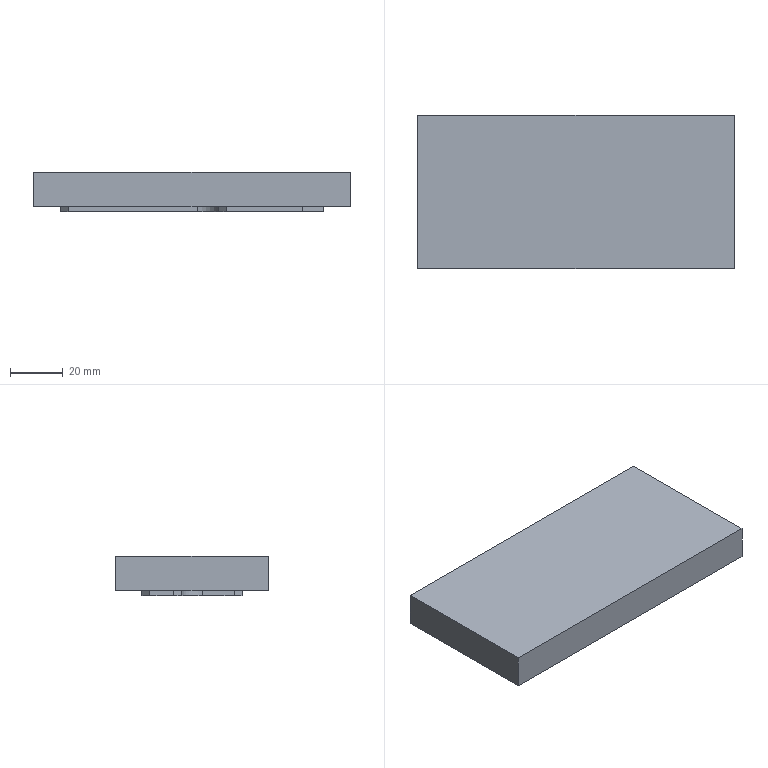NC program | NX | posted with a generic post | part box 120 x 58 x 15 mm
Lines 3611 to 3687 of 3687:
(11_COPY_COPY , TOOL : D6A45)
N7190 T01 M6
N7192 G54
N7194 G17 G0 G90 X30. Y0.741 S9500 M3
N7196 G43 Z30. H1
N7198 Z3.
N7200 G94 G1 Z-1. F1000.
N7202 X29.995
N7204 G3 X29.259 Y-0.005 R0.741
N7206 X30. Y0.741 R-0.741
N7208 X29.48 Y0.441 R0.6
N7210 G1 Z2.
N7212 G0 Z30.
N7214 X30. Y-14.791
N7216 Z3.
N7218 G1 Z-1.
N7220 G3 X44.791 Y0. R14.791
N7222 X30. Y14.791 R14.791
N7224 X29.209 Y14. R0.791
N7226 X30. Y13.209 R0.791
N7228 G2 X43.209 Y0. R13.209
N7230 X30. Y-13.209 R13.209
N7232 G3 X29.209 Y-14. R0.791
N7234 X30. Y-14.791 R0.791
N7236 X30.52 Y-14.491 R0.6
N7238 G1 Z2.
N7240 G0 Z30.
N7242 X6.042 Y13.081
N7244 Z2.
N7246 G1 Z-1.
N7248 X6.52 Y13.991
N7250 G3 X6. Y14.291 R0.6
N7252 G1 X-44.
N7254 G3 X-45.291 Y13. R1.291
N7256 X-44. Y11.709 R1.291
N7258 G1 X6.
N7260 G3 X7.291 Y13. R1.291
N7262 X6. Y14.291 R1.291
N7264 X5.48 Y13.991 R0.6
N7266 G1 X4.961 Y13.091
N7268 Z2.
N7270 G0 Z30.
N7272 X-47.921 Y20.952
N7274 Z2.
N7276 G1 Z-1.
N7278 X-47.52 Y20.259
N7280 G3 X-47.001 Y19.959 R0.6
N7282 G1 X42.001
N7284 G2 X42.677 Y19.678 R0.957
N7286 G1 X50.678 Y11.677
N7288 G2 X50.959 Y11. R0.957
N7290 G1 Y-11.
N7292 G2 X50.678 Y-11.677 R0.957
N7294 G1 X42.677 Y-19.678
N7296 G2 X42.001 Y-19.959 R0.957
N7298 G1 X12.999
N7300 G2 X12.323 Y-19.678 R0.957
N7302 G1 X9.322 Y-16.677
N7304 G2 X9.041 Y-16.001 R0.957
N7306 G1 Y-4.
N7308 G3 X2. Y3.041 R7.041
N7310 G1 X-47.001
N7312 G2 X-47.677 Y3.322 R0.957
N7314 G1 X-50.678 Y6.323
N7316 G2 X-50.959 Y6.999 R0.957
N7318 G1 Y16.001
N7320 G2 X-50.678 Y16.677 R0.957
N7322 G1 X-47.677 Y19.678
N7324 G2 X-47.001 Y19.959 R0.957
N7326 G3 X-46.481 Y20.259 R0.6
N7328 G1 X-45.961 Y21.159
N7330 Z2.
N7332 G0 Z30.
N7334 M5
N7336 M2